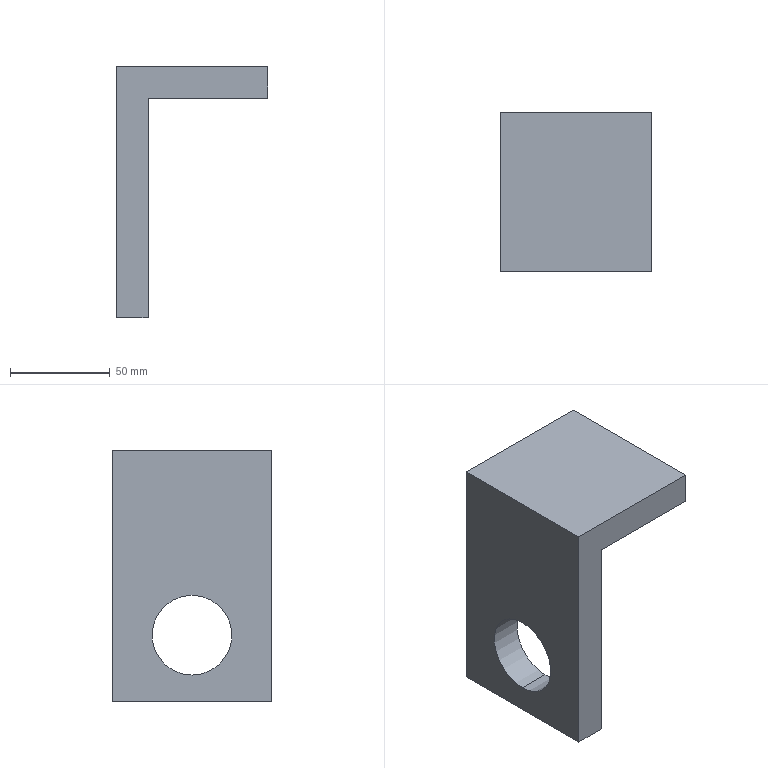Part | STEP file | PN_0017 Cylinder bracket | 1 solid | 10 faces | box 76 x 80 x 126 mm | volume 217974 mm3 | plane 8 | cylinder 2 | commonest cylinder face diameters 40 x2
STEP:
#1=CARTESIAN_POINT('',(0.,0.,0.));
#2=DIRECTION('',(0.,0.,1.));
#3=DIRECTION('',(1.,0.,0.));
#4=AXIS2_PLACEMENT_3D('',#1,#2,#3);
#5=CARTESIAN_POINT('',(-16.,40.,13.3));
#6=VERTEX_POINT('',#5);
#7=CARTESIAN_POINT('',(0.,40.,13.3));
#8=VERTEX_POINT('',#7);
#9=CARTESIAN_POINT('',(-80.,40.,13.3));
#10=DIRECTION('',(1.,0.,0.));
#11=VECTOR('',#10,1.);
#12=LINE('',#9,#11);
#13=CARTESIAN_POINT('',(-80.,40.,33.3));
#14=DIRECTION('',(1.,0.,0.));
#15=DIRECTION('',(0.,0.,-1.));
#16=AXIS2_PLACEMENT_3D('',#13,#14,#15);
#17=CYLINDRICAL_SURFACE('',#16,20.);
#18=CARTESIAN_POINT('',(6.283,0.));
#19=DIRECTION('',(0.,1.));
#20=VECTOR('',#19,1.);
#21=LINE('',#18,#20);
#22=(GEOMETRIC_REPRESENTATION_CONTEXT(2)PARAMETRIC_REPRESENTATION_CONTEXT()REPRESENTATION_CONTEXT('',''));
#23=DEFINITIONAL_REPRESENTATION('',(#21),#22);
#24=PCURVE('',#17,#23);
#25=CARTESIAN_POINT('',(-80.,40.,33.3));
#26=DIRECTION('',(1.,0.,0.));
#27=DIRECTION('',(0.,0.,-1.));
#28=AXIS2_PLACEMENT_3D('',#25,#26,#27);
#29=CYLINDRICAL_SURFACE('',#28,20.);
#30=CARTESIAN_POINT('',(0.,0.));
#31=DIRECTION('',(0.,1.));
#32=VECTOR('',#31,1.);
#33=LINE('',#30,#32);
#34=(GEOMETRIC_REPRESENTATION_CONTEXT(2)PARAMETRIC_REPRESENTATION_CONTEXT()REPRESENTATION_CONTEXT('',''));
#35=DEFINITIONAL_REPRESENTATION('',(#33),#34);
#36=PCURVE('',#29,#35);
#37=SURFACE_CURVE('',#12,(#24,#36),.PCURVE_S1.);
#38=EDGE_CURVE('',#6,#8,#37,.T.);
#39=ORIENTED_EDGE('',*,*,#38,.T.);
#40=CARTESIAN_POINT('',(0.,40.,53.3));
#41=VERTEX_POINT('',#40);
#42=CARTESIAN_POINT('',(0.,40.,33.3));
#43=DIRECTION('',(1.,0.,0.));
#44=DIRECTION('',(0.,0.,-1.));
#45=AXIS2_PLACEMENT_3D('',#42,#43,#44);
#46=CIRCLE('',#45,20.);
#47=CARTESIAN_POINT('',(0.,80.));
#48=DIRECTION('',(1.,0.));
#49=VECTOR('',#48,1.);
#50=LINE('',#47,#49);
#51=(GEOMETRIC_REPRESENTATION_CONTEXT(2)PARAMETRIC_REPRESENTATION_CONTEXT()REPRESENTATION_CONTEXT('',''));
#52=DEFINITIONAL_REPRESENTATION('',(#50),#51);
#53=PCURVE('',#17,#52);
#54=CARTESIAN_POINT('',(0.,80.,0.));
#55=DIRECTION('',(-1.,0.,0.));
#56=DIRECTION('',(0.,0.,1.));
#57=AXIS2_PLACEMENT_3D('',#54,#55,#56);
#58=PLANE('',#57);
#59=CARTESIAN_POINT('',(13.3,-40.));
#60=CARTESIAN_POINT('',(13.3,-5.359));
#61=CARTESIAN_POINT('',(43.3,-22.679));
#62=CARTESIAN_POINT('',(73.3,-40.));
#63=CARTESIAN_POINT('',(43.3,-57.321));
#64=CARTESIAN_POINT('',(13.3,-74.641));
#65=CARTESIAN_POINT('',(13.3,-40.));
#66=(BOUNDED_CURVE()B_SPLINE_CURVE(2,(#59,#60,#61,#62,#63,#64,#65),.UNSPECIFIED.,.T.,.F.)B_SPLINE_CURVE_WITH_KNOTS((1,2,2,2,2,1),(-2.094,0.,2.094,4.189,6.283,8.378),.UNSPECIFIED.)CURVE()GEOMETRIC_REPRESENTATION_ITEM()RATIONAL_B_SPLINE_CURVE((1.,0.5,1.,0.5,1.,0.5,1.))REPRESENTATION_ITEM(''));
#67=(GEOMETRIC_REPRESENTATION_CONTEXT(2)PARAMETRIC_REPRESENTATION_CONTEXT()REPRESENTATION_CONTEXT('',''));
#68=DEFINITIONAL_REPRESENTATION('',(#66),#67);
#69=PCURVE('',#58,#68);
#70=SURFACE_CURVE('',#46,(#53,#69),.PCURVE_S1.);
#71=EDGE_CURVE('',#41,#8,#70,.T.);
#72=ORIENTED_EDGE('',*,*,#71,.F.);
#73=CARTESIAN_POINT('',(-16.,40.,53.3));
#74=VERTEX_POINT('',#73);
#75=CARTESIAN_POINT('',(-80.,40.,53.3));
#76=DIRECTION('',(1.,0.,0.));
#77=VECTOR('',#76,1.);
#78=LINE('',#75,#77);
#79=CARTESIAN_POINT('',(3.142,0.));
#80=DIRECTION('',(0.,1.));
#81=VECTOR('',#80,1.);
#82=LINE('',#79,#81);
#83=(GEOMETRIC_REPRESENTATION_CONTEXT(2)PARAMETRIC_REPRESENTATION_CONTEXT()REPRESENTATION_CONTEXT('',''));
#84=DEFINITIONAL_REPRESENTATION('',(#82),#83);
#85=PCURVE('',#17,#84);
#86=CARTESIAN_POINT('',(3.142,0.));
#87=DIRECTION('',(0.,1.));
#88=VECTOR('',#87,1.);
#89=LINE('',#86,#88);
#90=(GEOMETRIC_REPRESENTATION_CONTEXT(2)PARAMETRIC_REPRESENTATION_CONTEXT()REPRESENTATION_CONTEXT('',''));
#91=DEFINITIONAL_REPRESENTATION('',(#89),#90);
#92=PCURVE('',#29,#91);
#93=SURFACE_CURVE('',#78,(#85,#92),.PCURVE_S1.);
#94=EDGE_CURVE('',#74,#41,#93,.T.);
#95=ORIENTED_EDGE('',*,*,#94,.F.);
#96=CARTESIAN_POINT('',(-16.,40.,33.3));
#97=DIRECTION('',(1.,0.,0.));
#98=DIRECTION('',(0.,0.,-1.));
#99=AXIS2_PLACEMENT_3D('',#96,#97,#98);
#100=CIRCLE('',#99,20.);
#101=CARTESIAN_POINT('',(0.,64.));
#102=DIRECTION('',(1.,0.));
#103=VECTOR('',#102,1.);
#104=LINE('',#101,#103);
#105=(GEOMETRIC_REPRESENTATION_CONTEXT(2)PARAMETRIC_REPRESENTATION_CONTEXT()REPRESENTATION_CONTEXT('',''));
#106=DEFINITIONAL_REPRESENTATION('',(#104),#105);
#107=PCURVE('',#17,#106);
#108=CARTESIAN_POINT('',(-16.,80.,0.));
#109=DIRECTION('',(1.,0.,0.));
#110=DIRECTION('',(0.,0.,-1.));
#111=AXIS2_PLACEMENT_3D('',#108,#109,#110);
#112=PLANE('',#111);
#113=CARTESIAN_POINT('',(-33.3,-40.));
#114=DIRECTION('',(1.,0.));
#115=AXIS2_PLACEMENT_2D('',#113,#114);
#116=CIRCLE('',#115,20.);
#117=(GEOMETRIC_REPRESENTATION_CONTEXT(2)PARAMETRIC_REPRESENTATION_CONTEXT()REPRESENTATION_CONTEXT('',''));
#118=DEFINITIONAL_REPRESENTATION('',(#116),#117);
#119=PCURVE('',#112,#118);
#120=SURFACE_CURVE('',#100,(#107,#119),.PCURVE_S1.);
#121=EDGE_CURVE('',#74,#6,#120,.T.);
#122=ORIENTED_EDGE('',*,*,#121,.T.);
#123=EDGE_LOOP('',(#39,#72,#95,#122));
#124=FACE_BOUND('',#123,.F.);
#125=ADVANCED_FACE('',(#124),#17,.F.);
#126=CARTESIAN_POINT('',(0.,0.,0.));
#127=VERTEX_POINT('',#126);
#128=CARTESIAN_POINT('',(-16.,0.,0.));
#129=VERTEX_POINT('',#128);
#130=CARTESIAN_POINT('',(-16.,0.,0.));
#131=DIRECTION('',(-1.,0.,0.));
#132=VECTOR('',#131,1.);
#133=LINE('',#130,#132);
#134=CARTESIAN_POINT('',(-16.,80.,0.));
#135=DIRECTION('',(0.,0.,1.));
#136=DIRECTION('',(1.,0.,0.));
#137=AXIS2_PLACEMENT_3D('',#134,#135,#136);
#138=PLANE('',#137);
#139=CARTESIAN_POINT('',(0.,-80.));
#140=DIRECTION('',(-1.,0.));
#141=VECTOR('',#140,1.);
#142=LINE('',#139,#141);
#143=(GEOMETRIC_REPRESENTATION_CONTEXT(2)PARAMETRIC_REPRESENTATION_CONTEXT()REPRESENTATION_CONTEXT('',''));
#144=DEFINITIONAL_REPRESENTATION('',(#142),#143);
#145=PCURVE('',#138,#144);
#146=CARTESIAN_POINT('',(0.,0.,0.));
#147=DIRECTION('',(0.,-1.,0.));
#148=DIRECTION('',(0.,0.,-1.));
#149=AXIS2_PLACEMENT_3D('',#146,#147,#148);
#150=PLANE('',#149);
#151=CARTESIAN_POINT('',(0.,-16.));
#152=DIRECTION('',(0.,-1.));
#153=VECTOR('',#152,1.);
#154=LINE('',#151,#153);
#155=(GEOMETRIC_REPRESENTATION_CONTEXT(2)PARAMETRIC_REPRESENTATION_CONTEXT()REPRESENTATION_CONTEXT('',''));
#156=DEFINITIONAL_REPRESENTATION('',(#154),#155);
#157=PCURVE('',#150,#156);
#158=SURFACE_CURVE('',#133,(#145,#157),.PCURVE_S1.);
#159=EDGE_CURVE('',#127,#129,#158,.T.);
#160=ORIENTED_EDGE('',*,*,#159,.T.);
#161=CARTESIAN_POINT('',(-16.,80.,0.));
#162=VERTEX_POINT('',#161);
#163=CARTESIAN_POINT('',(-16.,80.,0.));
#164=DIRECTION('',(0.,-1.,0.));
#165=VECTOR('',#164,1.);
#166=LINE('',#163,#165);
#167=CARTESIAN_POINT('',(0.,0.));
#168=DIRECTION('',(0.,-1.));
#169=VECTOR('',#168,1.);
#170=LINE('',#167,#169);
#171=(GEOMETRIC_REPRESENTATION_CONTEXT(2)PARAMETRIC_REPRESENTATION_CONTEXT()REPRESENTATION_CONTEXT('',''));
#172=DEFINITIONAL_REPRESENTATION('',(#170),#171);
#173=PCURVE('',#138,#172);
#174=CARTESIAN_POINT('',(0.,0.));
#175=DIRECTION('',(0.,-1.));
#176=VECTOR('',#175,1.);
#177=LINE('',#174,#176);
#178=(GEOMETRIC_REPRESENTATION_CONTEXT(2)PARAMETRIC_REPRESENTATION_CONTEXT()REPRESENTATION_CONTEXT('',''));
#179=DEFINITIONAL_REPRESENTATION('',(#177),#178);
#180=PCURVE('',#112,#179);
#181=SURFACE_CURVE('',#166,(#173,#180),.PCURVE_S1.);
#182=EDGE_CURVE('',#162,#129,#181,.T.);
#183=ORIENTED_EDGE('',*,*,#182,.F.);
#184=CARTESIAN_POINT('',(0.,80.,0.));
#185=VERTEX_POINT('',#184);
#186=CARTESIAN_POINT('',(-16.,80.,0.));
#187=DIRECTION('',(-1.,0.,0.));
#188=VECTOR('',#187,1.);
#189=LINE('',#186,#188);
#190=CARTESIAN_POINT('',(0.,0.));
#191=DIRECTION('',(-1.,0.));
#192=VECTOR('',#191,1.);
#193=LINE('',#190,#192);
#194=(GEOMETRIC_REPRESENTATION_CONTEXT(2)PARAMETRIC_REPRESENTATION_CONTEXT()REPRESENTATION_CONTEXT('',''));
#195=DEFINITIONAL_REPRESENTATION('',(#193),#194);
#196=PCURVE('',#138,#195);
#197=CARTESIAN_POINT('',(0.,80.,0.));
#198=DIRECTION('',(0.,-1.,0.));
#199=DIRECTION('',(0.,0.,-1.));
#200=AXIS2_PLACEMENT_3D('',#197,#198,#199);
#201=PLANE('',#200);
#202=CARTESIAN_POINT('',(0.,-16.));
#203=DIRECTION('',(0.,-1.));
#204=VECTOR('',#203,1.);
#205=LINE('',#202,#204);
#206=(GEOMETRIC_REPRESENTATION_CONTEXT(2)PARAMETRIC_REPRESENTATION_CONTEXT()REPRESENTATION_CONTEXT('',''));
#207=DEFINITIONAL_REPRESENTATION('',(#205),#206);
#208=PCURVE('',#201,#207);
#209=SURFACE_CURVE('',#189,(#196,#208),.PCURVE_S1.);
#210=EDGE_CURVE('',#185,#162,#209,.T.);
#211=ORIENTED_EDGE('',*,*,#210,.F.);
#212=CARTESIAN_POINT('',(0.,80.,0.));
#213=DIRECTION('',(0.,-1.,0.));
#214=VECTOR('',#213,1.);
#215=LINE('',#212,#214);
#216=CARTESIAN_POINT('',(16.,0.));
#217=DIRECTION('',(0.,-1.));
#218=VECTOR('',#217,1.);
#219=LINE('',#216,#218);
#220=(GEOMETRIC_REPRESENTATION_CONTEXT(2)PARAMETRIC_REPRESENTATION_CONTEXT()REPRESENTATION_CONTEXT('',''));
#221=DEFINITIONAL_REPRESENTATION('',(#219),#220);
#222=PCURVE('',#138,#221);
#223=CARTESIAN_POINT('',(0.,0.));
#224=DIRECTION('',(0.,-1.));
#225=VECTOR('',#224,1.);
#226=LINE('',#223,#225);
#227=(GEOMETRIC_REPRESENTATION_CONTEXT(2)PARAMETRIC_REPRESENTATION_CONTEXT()REPRESENTATION_CONTEXT('',''));
#228=DEFINITIONAL_REPRESENTATION('',(#226),#227);
#229=PCURVE('',#58,#228);
#230=SURFACE_CURVE('',#215,(#222,#229),.PCURVE_S1.);
#231=EDGE_CURVE('',#185,#127,#230,.T.);
#232=ORIENTED_EDGE('',*,*,#231,.T.);
#233=EDGE_LOOP('',(#160,#183,#211,#232));
#234=FACE_BOUND('',#233,.T.);
#235=ADVANCED_FACE('',(#234),#138,.F.);
#236=CARTESIAN_POINT('',(-16.,40.,33.3));
#237=DIRECTION('',(1.,0.,0.));
#238=DIRECTION('',(0.,0.,-1.));
#239=AXIS2_PLACEMENT_3D('',#236,#237,#238);
#240=CIRCLE('',#239,20.);
#241=CARTESIAN_POINT('',(-33.3,-40.));
#242=DIRECTION('',(1.,0.));
#243=AXIS2_PLACEMENT_2D('',#241,#242);
#244=CIRCLE('',#243,20.);
#245=(GEOMETRIC_REPRESENTATION_CONTEXT(2)PARAMETRIC_REPRESENTATION_CONTEXT()REPRESENTATION_CONTEXT('',''));
#246=DEFINITIONAL_REPRESENTATION('',(#244),#245);
#247=PCURVE('',#112,#246);
#248=CARTESIAN_POINT('',(0.,64.));
#249=DIRECTION('',(1.,0.));
#250=VECTOR('',#249,1.);
#251=LINE('',#248,#250);
#252=(GEOMETRIC_REPRESENTATION_CONTEXT(2)PARAMETRIC_REPRESENTATION_CONTEXT()REPRESENTATION_CONTEXT('',''));
#253=DEFINITIONAL_REPRESENTATION('',(#251),#252);
#254=PCURVE('',#29,#253);
#255=SURFACE_CURVE('',#240,(#247,#254),.PCURVE_S1.);
#256=EDGE_CURVE('',#6,#74,#255,.T.);
#257=ORIENTED_EDGE('',*,*,#256,.T.);
#258=ORIENTED_EDGE('',*,*,#121,.T.);
#259=EDGE_LOOP('',(#257,#258));
#260=FACE_BOUND('',#259,.T.);
#261=CARTESIAN_POINT('',(-16.,0.,126.));
#262=VERTEX_POINT('',#261);
#263=CARTESIAN_POINT('',(-16.,0.,0.));
#264=DIRECTION('',(0.,0.,1.));
#265=VECTOR('',#264,1.);
#266=LINE('',#263,#265);
#267=CARTESIAN_POINT('',(0.,-80.));
#268=DIRECTION('',(-1.,0.));
#269=VECTOR('',#268,1.);
#270=LINE('',#267,#269);
#271=(GEOMETRIC_REPRESENTATION_CONTEXT(2)PARAMETRIC_REPRESENTATION_CONTEXT()REPRESENTATION_CONTEXT('',''));
#272=DEFINITIONAL_REPRESENTATION('',(#270),#271);
#273=PCURVE('',#112,#272);
#274=CARTESIAN_POINT('',(0.,-16.));
#275=DIRECTION('',(-1.,0.));
#276=VECTOR('',#275,1.);
#277=LINE('',#274,#276);
#278=(GEOMETRIC_REPRESENTATION_CONTEXT(2)PARAMETRIC_REPRESENTATION_CONTEXT()REPRESENTATION_CONTEXT('',''));
#279=DEFINITIONAL_REPRESENTATION('',(#277),#278);
#280=PCURVE('',#150,#279);
#281=SURFACE_CURVE('',#266,(#273,#280),.PCURVE_S1.);
#282=EDGE_CURVE('',#129,#262,#281,.T.);
#283=ORIENTED_EDGE('',*,*,#282,.T.);
#284=CARTESIAN_POINT('',(-16.,80.,126.));
#285=VERTEX_POINT('',#284);
#286=CARTESIAN_POINT('',(-16.,80.,126.));
#287=DIRECTION('',(0.,-1.,0.));
#288=VECTOR('',#287,1.);
#289=LINE('',#286,#288);
#290=CARTESIAN_POINT('',(-126.,0.));
#291=DIRECTION('',(0.,-1.));
#292=VECTOR('',#291,1.);
#293=LINE('',#290,#292);
#294=(GEOMETRIC_REPRESENTATION_CONTEXT(2)PARAMETRIC_REPRESENTATION_CONTEXT()REPRESENTATION_CONTEXT('',''));
#295=DEFINITIONAL_REPRESENTATION('',(#293),#294);
#296=PCURVE('',#112,#295);
#297=CARTESIAN_POINT('',(-16.,80.,126.));
#298=DIRECTION('',(0.,0.,-1.));
#299=DIRECTION('',(-1.,0.,0.));
#300=AXIS2_PLACEMENT_3D('',#297,#298,#299);
#301=PLANE('',#300);
#302=CARTESIAN_POINT('',(0.,0.));
#303=DIRECTION('',(0.,-1.));
#304=VECTOR('',#303,1.);
#305=LINE('',#302,#304);
#306=(GEOMETRIC_REPRESENTATION_CONTEXT(2)PARAMETRIC_REPRESENTATION_CONTEXT()REPRESENTATION_CONTEXT('',''));
#307=DEFINITIONAL_REPRESENTATION('',(#305),#306);
#308=PCURVE('',#301,#307);
#309=SURFACE_CURVE('',#289,(#296,#308),.PCURVE_S1.);
#310=EDGE_CURVE('',#285,#262,#309,.T.);
#311=ORIENTED_EDGE('',*,*,#310,.F.);
#312=CARTESIAN_POINT('',(-16.,80.,0.));
#313=DIRECTION('',(0.,0.,1.));
#314=VECTOR('',#313,1.);
#315=LINE('',#312,#314);
#316=CARTESIAN_POINT('',(0.,0.));
#317=DIRECTION('',(-1.,0.));
#318=VECTOR('',#317,1.);
#319=LINE('',#316,#318);
#320=(GEOMETRIC_REPRESENTATION_CONTEXT(2)PARAMETRIC_REPRESENTATION_CONTEXT()REPRESENTATION_CONTEXT('',''));
#321=DEFINITIONAL_REPRESENTATION('',(#319),#320);
#322=PCURVE('',#112,#321);
#323=CARTESIAN_POINT('',(0.,-16.));
#324=DIRECTION('',(-1.,0.));
#325=VECTOR('',#324,1.);
#326=LINE('',#323,#325);
#327=(GEOMETRIC_REPRESENTATION_CONTEXT(2)PARAMETRIC_REPRESENTATION_CONTEXT()REPRESENTATION_CONTEXT('',''));
#328=DEFINITIONAL_REPRESENTATION('',(#326),#327);
#329=PCURVE('',#201,#328);
#330=SURFACE_CURVE('',#315,(#322,#329),.PCURVE_S1.);
#331=EDGE_CURVE('',#162,#285,#330,.T.);
#332=ORIENTED_EDGE('',*,*,#331,.F.);
#333=ORIENTED_EDGE('',*,*,#182,.T.);
#334=EDGE_LOOP('',(#283,#311,#332,#333));
#335=FACE_BOUND('',#334,.T.);
#336=ADVANCED_FACE('',(#260,#335),#112,.F.);
#337=CARTESIAN_POINT('',(60.,0.,126.));
#338=VERTEX_POINT('',#337);
#339=CARTESIAN_POINT('',(-16.,0.,126.));
#340=DIRECTION('',(1.,0.,0.));
#341=VECTOR('',#340,1.);
#342=LINE('',#339,#341);
#343=CARTESIAN_POINT('',(0.,-80.));
#344=DIRECTION('',(-1.,0.));
#345=VECTOR('',#344,1.);
#346=LINE('',#343,#345);
#347=(GEOMETRIC_REPRESENTATION_CONTEXT(2)PARAMETRIC_REPRESENTATION_CONTEXT()REPRESENTATION_CONTEXT('',''));
#348=DEFINITIONAL_REPRESENTATION('',(#346),#347);
#349=PCURVE('',#301,#348);
#350=CARTESIAN_POINT('',(-126.,-16.));
#351=DIRECTION('',(0.,1.));
#352=VECTOR('',#351,1.);
#353=LINE('',#350,#352);
#354=(GEOMETRIC_REPRESENTATION_CONTEXT(2)PARAMETRIC_REPRESENTATION_CONTEXT()REPRESENTATION_CONTEXT('',''));
#355=DEFINITIONAL_REPRESENTATION('',(#353),#354);
#356=PCURVE('',#150,#355);
#357=SURFACE_CURVE('',#342,(#349,#356),.PCURVE_S1.);
#358=EDGE_CURVE('',#262,#338,#357,.T.);
#359=ORIENTED_EDGE('',*,*,#358,.T.);
#360=CARTESIAN_POINT('',(60.,80.,126.));
#361=VERTEX_POINT('',#360);
#362=CARTESIAN_POINT('',(60.,80.,126.));
#363=DIRECTION('',(0.,-1.,0.));
#364=VECTOR('',#363,1.);
#365=LINE('',#362,#364);
#366=CARTESIAN_POINT('',(-76.,0.));
#367=DIRECTION('',(0.,-1.));
#368=VECTOR('',#367,1.);
#369=LINE('',#366,#368);
#370=(GEOMETRIC_REPRESENTATION_CONTEXT(2)PARAMETRIC_REPRESENTATION_CONTEXT()REPRESENTATION_CONTEXT('',''));
#371=DEFINITIONAL_REPRESENTATION('',(#369),#370);
#372=PCURVE('',#301,#371);
#373=CARTESIAN_POINT('',(60.,80.,110.));
#374=DIRECTION('',(-1.,0.,0.));
#375=DIRECTION('',(0.,0.,1.));
#376=AXIS2_PLACEMENT_3D('',#373,#374,#375);
#377=PLANE('',#376);
#378=CARTESIAN_POINT('',(16.,0.));
#379=DIRECTION('',(0.,-1.));
#380=VECTOR('',#379,1.);
#381=LINE('',#378,#380);
#382=(GEOMETRIC_REPRESENTATION_CONTEXT(2)PARAMETRIC_REPRESENTATION_CONTEXT()REPRESENTATION_CONTEXT('',''));
#383=DEFINITIONAL_REPRESENTATION('',(#381),#382);
#384=PCURVE('',#377,#383);
#385=SURFACE_CURVE('',#365,(#372,#384),.PCURVE_S1.);
#386=EDGE_CURVE('',#361,#338,#385,.T.);
#387=ORIENTED_EDGE('',*,*,#386,.F.);
#388=CARTESIAN_POINT('',(-16.,80.,126.));
#389=DIRECTION('',(1.,0.,0.));
#390=VECTOR('',#389,1.);
#391=LINE('',#388,#390);
#392=CARTESIAN_POINT('',(0.,0.));
#393=DIRECTION('',(-1.,0.));
#394=VECTOR('',#393,1.);
#395=LINE('',#392,#394);
#396=(GEOMETRIC_REPRESENTATION_CONTEXT(2)PARAMETRIC_REPRESENTATION_CONTEXT()REPRESENTATION_CONTEXT('',''));
#397=DEFINITIONAL_REPRESENTATION('',(#395),#396);
#398=PCURVE('',#301,#397);
#399=CARTESIAN_POINT('',(-126.,-16.));
#400=DIRECTION('',(0.,1.));
#401=VECTOR('',#400,1.);
#402=LINE('',#399,#401);
#403=(GEOMETRIC_REPRESENTATION_CONTEXT(2)PARAMETRIC_REPRESENTATION_CONTEXT()REPRESENTATION_CONTEXT('',''));
#404=DEFINITIONAL_REPRESENTATION('',(#402),#403);
#405=PCURVE('',#201,#404);
#406=SURFACE_CURVE('',#391,(#398,#405),.PCURVE_S1.);
#407=EDGE_CURVE('',#285,#361,#406,.T.);
#408=ORIENTED_EDGE('',*,*,#407,.F.);
#409=ORIENTED_EDGE('',*,*,#310,.T.);
#410=EDGE_LOOP('',(#359,#387,#408,#409));
#411=FACE_BOUND('',#410,.T.);
#412=ADVANCED_FACE('',(#411),#301,.F.);
#413=CARTESIAN_POINT('',(60.,0.,110.));
#414=VERTEX_POINT('',#413);
#415=CARTESIAN_POINT('',(60.,0.,110.));
#416=DIRECTION('',(0.,0.,-1.));
#417=VECTOR('',#416,1.);
#418=LINE('',#415,#417);
#419=CARTESIAN_POINT('',(0.,-80.));
#420=DIRECTION('',(-1.,0.));
#421=VECTOR('',#420,1.);
#422=LINE('',#419,#421);
#423=(GEOMETRIC_REPRESENTATION_CONTEXT(2)PARAMETRIC_REPRESENTATION_CONTEXT()REPRESENTATION_CONTEXT('',''));
#424=DEFINITIONAL_REPRESENTATION('',(#422),#423);
#425=PCURVE('',#377,#424);
#426=CARTESIAN_POINT('',(-110.,60.));
#427=DIRECTION('',(1.,0.));
#428=VECTOR('',#427,1.);
#429=LINE('',#426,#428);
#430=(GEOMETRIC_REPRESENTATION_CONTEXT(2)PARAMETRIC_REPRESENTATION_CONTEXT()REPRESENTATION_CONTEXT('',''));
#431=DEFINITIONAL_REPRESENTATION('',(#429),#430);
#432=PCURVE('',#150,#431);
#433=SURFACE_CURVE('',#418,(#425,#432),.PCURVE_S1.);
#434=EDGE_CURVE('',#338,#414,#433,.T.);
#435=ORIENTED_EDGE('',*,*,#434,.T.);
#436=CARTESIAN_POINT('',(60.,80.,110.));
#437=VERTEX_POINT('',#436);
#438=CARTESIAN_POINT('',(60.,80.,110.));
#439=DIRECTION('',(0.,-1.,0.));
#440=VECTOR('',#439,1.);
#441=LINE('',#438,#440);
#442=CARTESIAN_POINT('',(0.,0.));
#443=DIRECTION('',(0.,-1.));
#444=VECTOR('',#443,1.);
#445=LINE('',#442,#444);
#446=(GEOMETRIC_REPRESENTATION_CONTEXT(2)PARAMETRIC_REPRESENTATION_CONTEXT()REPRESENTATION_CONTEXT('',''));
#447=DEFINITIONAL_REPRESENTATION('',(#445),#446);
#448=PCURVE('',#377,#447);
#449=CARTESIAN_POINT('',(0.,80.,110.));
#450=DIRECTION('',(0.,0.,1.));
#451=DIRECTION('',(1.,0.,0.));
#452=AXIS2_PLACEMENT_3D('',#449,#450,#451);
#453=PLANE('',#452);
#454=CARTESIAN_POINT('',(60.,0.));
#455=DIRECTION('',(0.,-1.));
#456=VECTOR('',#455,1.);
#457=LINE('',#454,#456);
#458=(GEOMETRIC_REPRESENTATION_CONTEXT(2)PARAMETRIC_REPRESENTATION_CONTEXT()REPRESENTATION_CONTEXT('',''));
#459=DEFINITIONAL_REPRESENTATION('',(#457),#458);
#460=PCURVE('',#453,#459);
#461=SURFACE_CURVE('',#441,(#448,#460),.PCURVE_S1.);
#462=EDGE_CURVE('',#437,#414,#461,.T.);
#463=ORIENTED_EDGE('',*,*,#462,.F.);
#464=CARTESIAN_POINT('',(60.,80.,110.));
#465=DIRECTION('',(0.,0.,-1.));
#466=VECTOR('',#465,1.);
#467=LINE('',#464,#466);
#468=CARTESIAN_POINT('',(0.,0.));
#469=DIRECTION('',(-1.,0.));
#470=VECTOR('',#469,1.);
#471=LINE('',#468,#470);
#472=(GEOMETRIC_REPRESENTATION_CONTEXT(2)PARAMETRIC_REPRESENTATION_CONTEXT()REPRESENTATION_CONTEXT('',''));
#473=DEFINITIONAL_REPRESENTATION('',(#471),#472);
#474=PCURVE('',#377,#473);
#475=CARTESIAN_POINT('',(-110.,60.));
#476=DIRECTION('',(1.,0.));
#477=VECTOR('',#476,1.);
#478=LINE('',#475,#477);
#479=(GEOMETRIC_REPRESENTATION_CONTEXT(2)PARAMETRIC_REPRESENTATION_CONTEXT()REPRESENTATION_CONTEXT('',''));
#480=DEFINITIONAL_REPRESENTATION('',(#478),#479);
#481=PCURVE('',#201,#480);
#482=SURFACE_CURVE('',#467,(#474,#481),.PCURVE_S1.);
#483=EDGE_CURVE('',#361,#437,#482,.T.);
#484=ORIENTED_EDGE('',*,*,#483,.F.);
#485=ORIENTED_EDGE('',*,*,#386,.T.);
#486=EDGE_LOOP('',(#435,#463,#484,#485));
#487=FACE_BOUND('',#486,.T.);
#488=ADVANCED_FACE('',(#487),#377,.F.);
#489=CARTESIAN_POINT('',(0.,0.,110.));
#490=VERTEX_POINT('',#489);
#491=CARTESIAN_POINT('',(0.,0.,110.));
#492=DIRECTION('',(-1.,0.,0.));
#493=VECTOR('',#492,1.);
#494=LINE('',#491,#493);
#495=CARTESIAN_POINT('',(0.,-80.));
#496=DIRECTION('',(-1.,0.));
#497=VECTOR('',#496,1.);
#498=LINE('',#495,#497);
#499=(GEOMETRIC_REPRESENTATION_CONTEXT(2)PARAMETRIC_REPRESENTATION_CONTEXT()REPRESENTATION_CONTEXT('',''));
#500=DEFINITIONAL_REPRESENTATION('',(#498),#499);
#501=PCURVE('',#453,#500);
#502=CARTESIAN_POINT('',(-110.,0.));
#503=DIRECTION('',(0.,-1.));
#504=VECTOR('',#503,1.);
#505=LINE('',#502,#504);
#506=(GEOMETRIC_REPRESENTATION_CONTEXT(2)PARAMETRIC_REPRESENTATION_CONTEXT()REPRESENTATION_CONTEXT('',''));
#507=DEFINITIONAL_REPRESENTATION('',(#505),#506);
#508=PCURVE('',#150,#507);
#509=SURFACE_CURVE('',#494,(#501,#508),.PCURVE_S1.);
#510=EDGE_CURVE('',#414,#490,#509,.T.);
#511=ORIENTED_EDGE('',*,*,#510,.T.);
#512=CARTESIAN_POINT('',(0.,80.,110.));
#513=VERTEX_POINT('',#512);
#514=CARTESIAN_POINT('',(0.,80.,110.));
#515=DIRECTION('',(0.,-1.,0.));
#516=VECTOR('',#515,1.);
#517=LINE('',#514,#516);
#518=CARTESIAN_POINT('',(0.,0.));
#519=DIRECTION('',(0.,-1.));
#520=VECTOR('',#519,1.);
#521=LINE('',#518,#520);
#522=(GEOMETRIC_REPRESENTATION_CONTEXT(2)PARAMETRIC_REPRESENTATION_CONTEXT()REPRESENTATION_CONTEXT('',''));
#523=DEFINITIONAL_REPRESENTATION('',(#521),#522);
#524=PCURVE('',#453,#523);
#525=CARTESIAN_POINT('',(110.,0.));
#526=DIRECTION('',(0.,-1.));
#527=VECTOR('',#526,1.);
#528=LINE('',#525,#527);
#529=(GEOMETRIC_REPRESENTATION_CONTEXT(2)PARAMETRIC_REPRESENTATION_CONTEXT()REPRESENTATION_CONTEXT('',''));
#530=DEFINITIONAL_REPRESENTATION('',(#528),#529);
#531=PCURVE('',#58,#530);
#532=SURFACE_CURVE('',#517,(#524,#531),.PCURVE_S1.);
#533=EDGE_CURVE('',#513,#490,#532,.T.);
#534=ORIENTED_EDGE('',*,*,#533,.F.);
#535=CARTESIAN_POINT('',(0.,80.,110.));
#536=DIRECTION('',(-1.,0.,0.));
#537=VECTOR('',#536,1.);
#538=LINE('',#535,#537);
#539=CARTESIAN_POINT('',(0.,0.));
#540=DIRECTION('',(-1.,0.));
#541=VECTOR('',#540,1.);
#542=LINE('',#539,#541);
#543=(GEOMETRIC_REPRESENTATION_CONTEXT(2)PARAMETRIC_REPRESENTATION_CONTEXT()REPRESENTATION_CONTEXT('',''));
#544=DEFINITIONAL_REPRESENTATION('',(#542),#543);
#545=PCURVE('',#453,#544);
#546=CARTESIAN_POINT('',(-110.,0.));
#547=DIRECTION('',(0.,-1.));
#548=VECTOR('',#547,1.);
#549=LINE('',#546,#548);
#550=(GEOMETRIC_REPRESENTATION_CONTEXT(2)PARAMETRIC_REPRESENTATION_CONTEXT()REPRESENTATION_CONTEXT('',''));
#551=DEFINITIONAL_REPRESENTATION('',(#549),#550);
#552=PCURVE('',#201,#551);
#553=SURFACE_CURVE('',#538,(#545,#552),.PCURVE_S1.);
#554=EDGE_CURVE('',#437,#513,#553,.T.);
#555=ORIENTED_EDGE('',*,*,#554,.F.);
#556=ORIENTED_EDGE('',*,*,#462,.T.);
#557=EDGE_LOOP('',(#511,#534,#555,#556));
#558=FACE_BOUND('',#557,.T.);
#559=ADVANCED_FACE('',(#558),#453,.F.);
#560=CARTESIAN_POINT('',(0.,40.,33.3));
#561=DIRECTION('',(1.,0.,0.));
#562=DIRECTION('',(0.,0.,-1.));
#563=AXIS2_PLACEMENT_3D('',#560,#561,#562);
#564=CIRCLE('',#563,20.);
#565=CARTESIAN_POINT('',(13.3,-40.));
#566=CARTESIAN_POINT('',(13.3,-5.359));
#567=CARTESIAN_POINT('',(43.3,-22.679));
#568=CARTESIAN_POINT('',(73.3,-40.));
#569=CARTESIAN_POINT('',(43.3,-57.321));
#570=CARTESIAN_POINT('',(13.3,-74.641));
#571=CARTESIAN_POINT('',(13.3,-40.));
#572=(BOUNDED_CURVE()B_SPLINE_CURVE(2,(#565,#566,#567,#568,#569,#570,#571),.UNSPECIFIED.,.T.,.F.)B_SPLINE_CURVE_WITH_KNOTS((1,2,2,2,2,1),(-2.094,0.,2.094,4.189,6.283,8.378),.UNSPECIFIED.)CURVE()GEOMETRIC_REPRESENTATION_ITEM()RATIONAL_B_SPLINE_CURVE((1.,0.5,1.,0.5,1.,0.5,1.))REPRESENTATION_ITEM(''));
#573=(GEOMETRIC_REPRESENTATION_CONTEXT(2)PARAMETRIC_REPRESENTATION_CONTEXT()REPRESENTATION_CONTEXT('',''));
#574=DEFINITIONAL_REPRESENTATION('',(#572),#573);
#575=PCURVE('',#58,#574);
#576=CARTESIAN_POINT('',(0.,80.));
#577=DIRECTION('',(1.,0.));
#578=VECTOR('',#577,1.);
#579=LINE('',#576,#578);
#580=(GEOMETRIC_REPRESENTATION_CONTEXT(2)PARAMETRIC_REPRESENTATION_CONTEXT()REPRESENTATION_CONTEXT('',''));
#581=DEFINITIONAL_REPRESENTATION('',(#579),#580);
#582=PCURVE('',#29,#581);
#583=SURFACE_CURVE('',#564,(#575,#582),.PCURVE_S1.);
#584=EDGE_CURVE('',#8,#41,#583,.T.);
#585=ORIENTED_EDGE('',*,*,#584,.F.);
#586=ORIENTED_EDGE('',*,*,#71,.F.);
#587=EDGE_LOOP('',(#585,#586));
#588=FACE_BOUND('',#587,.T.);
#589=CARTESIAN_POINT('',(0.,0.,0.));
#590=DIRECTION('',(0.,0.,-1.));
#591=VECTOR('',#590,1.);
#592=LINE('',#589,#591);
#593=CARTESIAN_POINT('',(0.,-80.));
#594=DIRECTION('',(-1.,0.));
#595=VECTOR('',#594,1.);
#596=LINE('',#593,#595);
#597=(GEOMETRIC_REPRESENTATION_CONTEXT(2)PARAMETRIC_REPRESENTATION_CONTEXT()REPRESENTATION_CONTEXT('',''));
#598=DEFINITIONAL_REPRESENTATION('',(#596),#597);
#599=PCURVE('',#58,#598);
#600=CARTESIAN_POINT('',(0.,0.));
#601=DIRECTION('',(1.,0.));
#602=VECTOR('',#601,1.);
#603=LINE('',#600,#602);
#604=(GEOMETRIC_REPRESENTATION_CONTEXT(2)PARAMETRIC_REPRESENTATION_CONTEXT()REPRESENTATION_CONTEXT('',''));
#605=DEFINITIONAL_REPRESENTATION('',(#603),#604);
#606=PCURVE('',#150,#605);
#607=SURFACE_CURVE('',#592,(#599,#606),.PCURVE_S1.);
#608=EDGE_CURVE('',#490,#127,#607,.T.);
#609=ORIENTED_EDGE('',*,*,#608,.T.);
#610=ORIENTED_EDGE('',*,*,#231,.F.);
#611=CARTESIAN_POINT('',(0.,80.,0.));
#612=DIRECTION('',(0.,0.,-1.));
#613=VECTOR('',#612,1.);
#614=LINE('',#611,#613);
#615=CARTESIAN_POINT('',(0.,0.));
#616=DIRECTION('',(-1.,0.));
#617=VECTOR('',#616,1.);
#618=LINE('',#615,#617);
#619=(GEOMETRIC_REPRESENTATION_CONTEXT(2)PARAMETRIC_REPRESENTATION_CONTEXT()REPRESENTATION_CONTEXT('',''));
#620=DEFINITIONAL_REPRESENTATION('',(#618),#619);
#621=PCURVE('',#58,#620);
#622=CARTESIAN_POINT('',(0.,0.));
#623=DIRECTION('',(1.,0.));
#624=VECTOR('',#623,1.);
#625=LINE('',#622,#624);
#626=(GEOMETRIC_REPRESENTATION_CONTEXT(2)PARAMETRIC_REPRESENTATION_CONTEXT()REPRESENTATION_CONTEXT('',''));
#627=DEFINITIONAL_REPRESENTATION('',(#625),#626);
#628=PCURVE('',#201,#627);
#629=SURFACE_CURVE('',#614,(#621,#628),.PCURVE_S1.);
#630=EDGE_CURVE('',#513,#185,#629,.T.);
#631=ORIENTED_EDGE('',*,*,#630,.F.);
#632=ORIENTED_EDGE('',*,*,#533,.T.);
#633=EDGE_LOOP('',(#609,#610,#631,#632));
#634=FACE_BOUND('',#633,.T.);
#635=ADVANCED_FACE('',(#588,#634),#58,.F.);
#636=ORIENTED_EDGE('',*,*,#210,.T.);
#637=ORIENTED_EDGE('',*,*,#331,.T.);
#638=ORIENTED_EDGE('',*,*,#407,.T.);
#639=ORIENTED_EDGE('',*,*,#483,.T.);
#640=ORIENTED_EDGE('',*,*,#554,.T.);
#641=ORIENTED_EDGE('',*,*,#630,.T.);
#642=EDGE_LOOP('',(#636,#637,#638,#639,#640,#641));
#643=FACE_BOUND('',#642,.T.);
#644=ADVANCED_FACE('',(#643),#201,.F.);
#645=ORIENTED_EDGE('',*,*,#159,.F.);
#646=ORIENTED_EDGE('',*,*,#608,.F.);
#647=ORIENTED_EDGE('',*,*,#510,.F.);
#648=ORIENTED_EDGE('',*,*,#434,.F.);
#649=ORIENTED_EDGE('',*,*,#358,.F.);
#650=ORIENTED_EDGE('',*,*,#282,.F.);
#651=EDGE_LOOP('',(#645,#646,#647,#648,#649,#650));
#652=FACE_BOUND('',#651,.T.);
#653=ADVANCED_FACE('',(#652),#150,.T.);
#654=ORIENTED_EDGE('',*,*,#584,.F.);
#655=ORIENTED_EDGE('',*,*,#38,.F.);
#656=ORIENTED_EDGE('',*,*,#256,.T.);
#657=ORIENTED_EDGE('',*,*,#94,.T.);
#658=EDGE_LOOP('',(#654,#655,#656,#657));
#659=FACE_BOUND('',#658,.F.);
#660=ADVANCED_FACE('',(#659),#29,.F.);
#661=CLOSED_SHELL('',(#125,#235,#336,#412,#488,#559,#635,#644,#653,#660));
#662=MANIFOLD_SOLID_BREP('',#661);
#663=(LENGTH_UNIT()NAMED_UNIT(*)SI_UNIT(.MILLI.,.METRE.));
#664=UNCERTAINTY_MEASURE_WITH_UNIT(LENGTH_MEASURE(0.0000001),#663,'','');
#665=(NAMED_UNIT(*)PLANE_ANGLE_UNIT()SI_UNIT($,.RADIAN.));
#666=(NAMED_UNIT(*)SI_UNIT($,.STERADIAN.)SOLID_ANGLE_UNIT());
#667=(GEOMETRIC_REPRESENTATION_CONTEXT(3)GLOBAL_UNCERTAINTY_ASSIGNED_CONTEXT((#664))GLOBAL_UNIT_ASSIGNED_CONTEXT((#663,#665,#666))REPRESENTATION_CONTEXT('',''));
#668=ADVANCED_BREP_SHAPE_REPRESENTATION('',(#4,#662),#667);